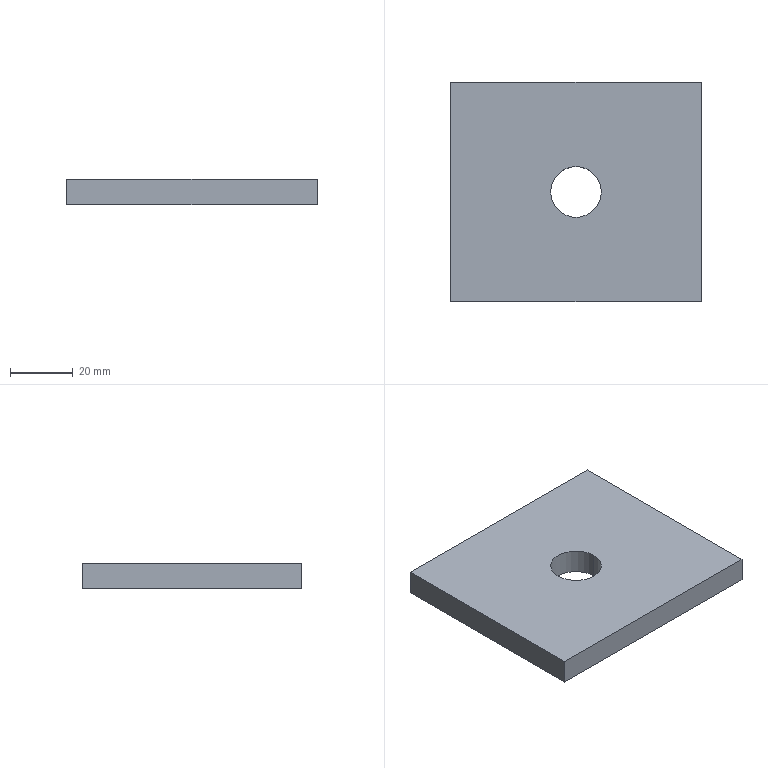Part | SolidWorks | features Extrusion 1, ICE 1 | 1 solid | 8 faces | box 80 x 70 x 8 mm | volume 43151 mm3 | plane 6 | cylinder 2 | commonest cylinder face diameters 16.2 x2
STEP:
#1=CARTESIAN_POINT('',(-8.1,0.,-4.));
#2=VERTEX_POINT('',#1);
#3=CARTESIAN_POINT('',(8.1,0.,-4.));
#4=VERTEX_POINT('',#3);
#5=CARTESIAN_POINT('',(0.,0.,-4.));
#6=DIRECTION('',(0.,0.,1.));
#7=DIRECTION('',(1.,0.,0.));
#8=AXIS2_PLACEMENT_3D('',#5,#6,#7);
#9=CIRCLE('',#8,8.1);
#10=EDGE_CURVE('',#2,#4,#9,.T.);
#11=ORIENTED_EDGE('',*,*,#10,.F.);
#12=CARTESIAN_POINT('',(-8.1,0.,4.));
#13=VERTEX_POINT('',#12);
#14=CARTESIAN_POINT('',(-8.1,0.,-14.));
#15=DIRECTION('',(0.,0.,1.));
#16=VECTOR('',#15,1000.);
#17=LINE('',#14,#16);
#18=EDGE_CURVE('',#2,#13,#17,.T.);
#19=ORIENTED_EDGE('',*,*,#18,.T.);
#20=CARTESIAN_POINT('',(8.1,0.,4.));
#21=VERTEX_POINT('',#20);
#22=CARTESIAN_POINT('',(0.,0.,4.));
#23=DIRECTION('',(0.,0.,1.));
#24=DIRECTION('',(1.,0.,0.));
#25=AXIS2_PLACEMENT_3D('',#22,#23,#24);
#26=CIRCLE('',#25,8.1);
#27=EDGE_CURVE('',#13,#21,#26,.T.);
#28=ORIENTED_EDGE('',*,*,#27,.T.);
#29=CARTESIAN_POINT('',(8.1,0.,-14.));
#30=DIRECTION('',(0.,0.,1.));
#31=VECTOR('',#30,1000.);
#32=LINE('',#29,#31);
#33=EDGE_CURVE('',#4,#21,#32,.T.);
#34=ORIENTED_EDGE('',*,*,#33,.F.);
#35=EDGE_LOOP('',(#11,#19,#28,#34));
#36=FACE_OUTER_BOUND('',#35,.T.);
#37=CARTESIAN_POINT('',(0.,0.,-14.));
#38=DIRECTION('',(0.,0.,1.));
#39=DIRECTION('',(1.,0.,0.));
#40=AXIS2_PLACEMENT_3D('',#37,#38,#39);
#41=CYLINDRICAL_SURFACE('',#40,8.1);
#42=ADVANCED_FACE('',(#36),#41,.F.);
#43=CARTESIAN_POINT('',(-40.,35.,4.));
#44=VERTEX_POINT('',#43);
#45=CARTESIAN_POINT('',(-40.,-35.,4.));
#46=VERTEX_POINT('',#45);
#47=CARTESIAN_POINT('',(-40.,35.,4.));
#48=DIRECTION('',(0.,-1.,0.));
#49=VECTOR('',#48,1000.);
#50=LINE('',#47,#49);
#51=EDGE_CURVE('',#44,#46,#50,.T.);
#52=ORIENTED_EDGE('',*,*,#51,.F.);
#53=CARTESIAN_POINT('',(-40.,35.,-4.));
#54=VERTEX_POINT('',#53);
#55=CARTESIAN_POINT('',(-40.,35.,-4.));
#56=DIRECTION('',(0.,0.,1.));
#57=VECTOR('',#56,1000.);
#58=LINE('',#55,#57);
#59=EDGE_CURVE('',#54,#44,#58,.T.);
#60=ORIENTED_EDGE('',*,*,#59,.F.);
#61=CARTESIAN_POINT('',(-40.,-35.,-4.));
#62=VERTEX_POINT('',#61);
#63=CARTESIAN_POINT('',(-40.,35.,-4.));
#64=DIRECTION('',(0.,-1.,0.));
#65=VECTOR('',#64,1000.);
#66=LINE('',#63,#65);
#67=EDGE_CURVE('',#54,#62,#66,.T.);
#68=ORIENTED_EDGE('',*,*,#67,.T.);
#69=CARTESIAN_POINT('',(-40.,-35.,-4.));
#70=DIRECTION('',(0.,0.,1.));
#71=VECTOR('',#70,1000.);
#72=LINE('',#69,#71);
#73=EDGE_CURVE('',#62,#46,#72,.T.);
#74=ORIENTED_EDGE('',*,*,#73,.T.);
#75=EDGE_LOOP('',(#52,#60,#68,#74));
#76=FACE_OUTER_BOUND('',#75,.T.);
#77=CARTESIAN_POINT('',(-40.,35.,-4.));
#78=DIRECTION('',(-1.,0.,0.));
#79=DIRECTION('',(0.,0.,1.));
#80=AXIS2_PLACEMENT_3D('',#77,#78,#79);
#81=PLANE('',#80);
#82=ADVANCED_FACE('',(#76),#81,.T.);
#83=CARTESIAN_POINT('',(40.,35.,4.));
#84=VERTEX_POINT('',#83);
#85=CARTESIAN_POINT('',(40.,35.,4.));
#86=DIRECTION('',(-1.,0.,0.));
#87=VECTOR('',#86,1000.);
#88=LINE('',#85,#87);
#89=EDGE_CURVE('',#84,#44,#88,.T.);
#90=ORIENTED_EDGE('',*,*,#89,.F.);
#91=CARTESIAN_POINT('',(40.,35.,-4.));
#92=VERTEX_POINT('',#91);
#93=CARTESIAN_POINT('',(40.,35.,-4.));
#94=DIRECTION('',(0.,0.,1.));
#95=VECTOR('',#94,1000.);
#96=LINE('',#93,#95);
#97=EDGE_CURVE('',#92,#84,#96,.T.);
#98=ORIENTED_EDGE('',*,*,#97,.F.);
#99=CARTESIAN_POINT('',(40.,35.,-4.));
#100=DIRECTION('',(-1.,0.,0.));
#101=VECTOR('',#100,1000.);
#102=LINE('',#99,#101);
#103=EDGE_CURVE('',#92,#54,#102,.T.);
#104=ORIENTED_EDGE('',*,*,#103,.T.);
#105=ORIENTED_EDGE('',*,*,#59,.T.);
#106=EDGE_LOOP('',(#90,#98,#104,#105));
#107=FACE_OUTER_BOUND('',#106,.T.);
#108=CARTESIAN_POINT('',(40.,35.,-4.));
#109=DIRECTION('',(0.,1.,0.));
#110=DIRECTION('',(0.,0.,1.));
#111=AXIS2_PLACEMENT_3D('',#108,#109,#110);
#112=PLANE('',#111);
#113=ADVANCED_FACE('',(#107),#112,.T.);
#114=CARTESIAN_POINT('',(40.,-35.,4.));
#115=VERTEX_POINT('',#114);
#116=CARTESIAN_POINT('',(40.,-35.,4.));
#117=DIRECTION('',(0.,1.,0.));
#118=VECTOR('',#117,1000.);
#119=LINE('',#116,#118);
#120=EDGE_CURVE('',#115,#84,#119,.T.);
#121=ORIENTED_EDGE('',*,*,#120,.F.);
#122=CARTESIAN_POINT('',(40.,-35.,-4.));
#123=VERTEX_POINT('',#122);
#124=CARTESIAN_POINT('',(40.,-35.,-4.));
#125=DIRECTION('',(0.,0.,1.));
#126=VECTOR('',#125,1000.);
#127=LINE('',#124,#126);
#128=EDGE_CURVE('',#123,#115,#127,.T.);
#129=ORIENTED_EDGE('',*,*,#128,.F.);
#130=CARTESIAN_POINT('',(40.,-35.,-4.));
#131=DIRECTION('',(0.,1.,0.));
#132=VECTOR('',#131,1000.);
#133=LINE('',#130,#132);
#134=EDGE_CURVE('',#123,#92,#133,.T.);
#135=ORIENTED_EDGE('',*,*,#134,.T.);
#136=ORIENTED_EDGE('',*,*,#97,.T.);
#137=EDGE_LOOP('',(#121,#129,#135,#136));
#138=FACE_OUTER_BOUND('',#137,.T.);
#139=CARTESIAN_POINT('',(40.,-35.,-4.));
#140=DIRECTION('',(1.,0.,0.));
#141=DIRECTION('',(0.,0.,-1.));
#142=AXIS2_PLACEMENT_3D('',#139,#140,#141);
#143=PLANE('',#142);
#144=ADVANCED_FACE('',(#138),#143,.T.);
#145=CARTESIAN_POINT('',(-40.,-35.,4.));
#146=DIRECTION('',(1.,0.,0.));
#147=VECTOR('',#146,1000.);
#148=LINE('',#145,#147);
#149=EDGE_CURVE('',#46,#115,#148,.T.);
#150=ORIENTED_EDGE('',*,*,#149,.F.);
#151=ORIENTED_EDGE('',*,*,#73,.F.);
#152=CARTESIAN_POINT('',(-40.,-35.,-4.));
#153=DIRECTION('',(1.,0.,0.));
#154=VECTOR('',#153,1000.);
#155=LINE('',#152,#154);
#156=EDGE_CURVE('',#62,#123,#155,.T.);
#157=ORIENTED_EDGE('',*,*,#156,.T.);
#158=ORIENTED_EDGE('',*,*,#128,.T.);
#159=EDGE_LOOP('',(#150,#151,#157,#158));
#160=FACE_OUTER_BOUND('',#159,.T.);
#161=CARTESIAN_POINT('',(-40.,-35.,-4.));
#162=DIRECTION('',(0.,-1.,0.));
#163=DIRECTION('',(0.,0.,-1.));
#164=AXIS2_PLACEMENT_3D('',#161,#162,#163);
#165=PLANE('',#164);
#166=ADVANCED_FACE('',(#160),#165,.T.);
#167=CARTESIAN_POINT('',(0.,0.,-4.));
#168=DIRECTION('',(0.,0.,1.));
#169=DIRECTION('',(1.,0.,0.));
#170=AXIS2_PLACEMENT_3D('',#167,#168,#169);
#171=CIRCLE('',#170,8.1);
#172=EDGE_CURVE('',#4,#2,#171,.T.);
#173=ORIENTED_EDGE('',*,*,#172,.T.);
#174=ORIENTED_EDGE('',*,*,#10,.T.);
#175=EDGE_LOOP('',(#173,#174));
#176=FACE_BOUND('',#175,.T.);
#177=ORIENTED_EDGE('',*,*,#67,.F.);
#178=ORIENTED_EDGE('',*,*,#103,.F.);
#179=ORIENTED_EDGE('',*,*,#134,.F.);
#180=ORIENTED_EDGE('',*,*,#156,.F.);
#181=EDGE_LOOP('',(#177,#178,#179,#180));
#182=FACE_OUTER_BOUND('',#181,.T.);
#183=CARTESIAN_POINT('',(0.,0.,-4.));
#184=DIRECTION('',(0.,0.,1.));
#185=DIRECTION('',(1.,0.,0.));
#186=AXIS2_PLACEMENT_3D('',#183,#184,#185);
#187=PLANE('',#186);
#188=ADVANCED_FACE('',(#176,#182),#187,.F.);
#189=CARTESIAN_POINT('',(0.,0.,4.));
#190=DIRECTION('',(0.,0.,1.));
#191=DIRECTION('',(1.,0.,0.));
#192=AXIS2_PLACEMENT_3D('',#189,#190,#191);
#193=CIRCLE('',#192,8.1);
#194=EDGE_CURVE('',#21,#13,#193,.T.);
#195=ORIENTED_EDGE('',*,*,#194,.F.);
#196=ORIENTED_EDGE('',*,*,#27,.F.);
#197=EDGE_LOOP('',(#195,#196));
#198=FACE_BOUND('',#197,.T.);
#199=ORIENTED_EDGE('',*,*,#51,.T.);
#200=ORIENTED_EDGE('',*,*,#149,.T.);
#201=ORIENTED_EDGE('',*,*,#120,.T.);
#202=ORIENTED_EDGE('',*,*,#89,.T.);
#203=EDGE_LOOP('',(#199,#200,#201,#202));
#204=FACE_OUTER_BOUND('',#203,.T.);
#205=CARTESIAN_POINT('',(0.,0.,4.));
#206=DIRECTION('',(0.,0.,1.));
#207=DIRECTION('',(1.,0.,0.));
#208=AXIS2_PLACEMENT_3D('',#205,#206,#207);
#209=PLANE('',#208);
#210=ADVANCED_FACE('',(#198,#204),#209,.T.);
#211=ORIENTED_EDGE('',*,*,#18,.F.);
#212=ORIENTED_EDGE('',*,*,#172,.F.);
#213=ORIENTED_EDGE('',*,*,#33,.T.);
#214=ORIENTED_EDGE('',*,*,#194,.T.);
#215=EDGE_LOOP('',(#211,#212,#213,#214));
#216=FACE_OUTER_BOUND('',#215,.T.);
#217=CARTESIAN_POINT('',(0.,0.,-14.));
#218=DIRECTION('',(0.,0.,1.));
#219=DIRECTION('',(1.,0.,0.));
#220=AXIS2_PLACEMENT_3D('',#217,#218,#219);
#221=CYLINDRICAL_SURFACE('',#220,8.1);
#222=ADVANCED_FACE('',(#216),#221,.F.);
#223=CLOSED_SHELL('',(#42,#82,#113,#144,#166,#188,#210,#222));
#224=MANIFOLD_SOLID_BREP('',#223);
#225=CARTESIAN_POINT('',(0.,0.,0.));
#226=DIRECTION('',(0.,0.,1.));
#227=DIRECTION('',(1.,0.,0.));
#228=AXIS2_PLACEMENT_3D('',#225,#226,#227);
#229=(LENGTH_UNIT()NAMED_UNIT(*)SI_UNIT(.MILLI.,.METRE.));
#230=UNCERTAINTY_MEASURE_WITH_UNIT(LENGTH_MEASURE(0.00001),#229,'','');
#231=(NAMED_UNIT(*)PLANE_ANGLE_UNIT()SI_UNIT($,.RADIAN.));
#232=(NAMED_UNIT(*)SI_UNIT($,.STERADIAN.)SOLID_ANGLE_UNIT());
#233=(GEOMETRIC_REPRESENTATION_CONTEXT(3)GLOBAL_UNCERTAINTY_ASSIGNED_CONTEXT((#230))GLOBAL_UNIT_ASSIGNED_CONTEXT((#229,#231,#232))REPRESENTATION_CONTEXT('',''));
#234=ADVANCED_BREP_SHAPE_REPRESENTATION('',(#224,#228),#233);